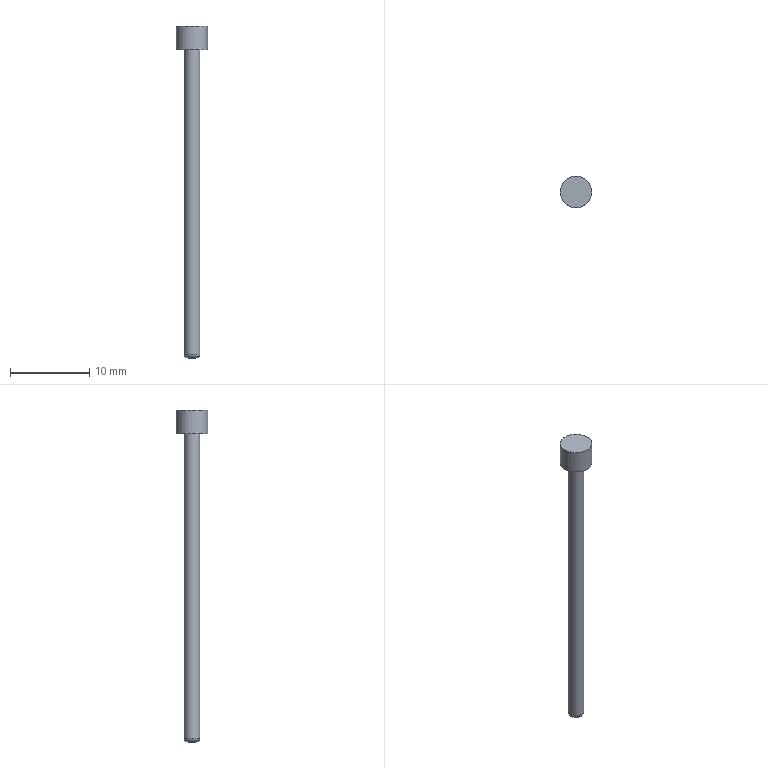Part | STEP file | gslz 2016.10.28-10_id2602_x_t | 1 solid | 6 faces | box 4 x 4 x 42 mm | volume 159.922 mm3 | plane 3 | cylinder 2 | torus 1 | commonest cylinder face diameters 2 x1 4 x1
STEP:
#1=CARTESIAN_POINT('',(0.,0.,0.));
#2=DIRECTION('',(0.,0.,1.));
#3=DIRECTION('',(1.,0.,0.));
#4=AXIS2_PLACEMENT_3D('',#1,#2,#3);
#5=CARTESIAN_POINT('',(1162.303,113.3,-12.5));
#6=VERTEX_POINT('',#5);
#7=CARTESIAN_POINT('',(1161.303,113.3,-12.5));
#8=DIRECTION('',(0.,0.,1.));
#9=DIRECTION('',(1.,0.,0.));
#10=AXIS2_PLACEMENT_3D('',#7,#8,#9);
#11=CIRCLE('',#10,1.);
#12=CARTESIAN_POINT('',(1161.303,113.3,-13.));
#13=DIRECTION('',(0.,0.,1.));
#14=DIRECTION('',(-1.,0.,0.));
#15=AXIS2_PLACEMENT_3D('',#12,#13,#14);
#16=CYLINDRICAL_SURFACE('',#15,1.);
#17=CARTESIAN_POINT('',(3.142,0.5));
#18=DIRECTION('',(1.,0.));
#19=VECTOR('',#18,1.);
#20=LINE('',#17,#19);
#21=(GEOMETRIC_REPRESENTATION_CONTEXT(2)PARAMETRIC_REPRESENTATION_CONTEXT()REPRESENTATION_CONTEXT('',''));
#22=DEFINITIONAL_REPRESENTATION('',(#20),#21);
#23=PCURVE('',#16,#22);
#24=CARTESIAN_POINT('',(1161.303,113.3,-12.5));
#25=DIRECTION('',(0.,0.,1.));
#26=DIRECTION('',(0.,-1.,0.));
#27=AXIS2_PLACEMENT_3D('',#24,#25,#26);
#28=TOROIDAL_SURFACE('',#27,0.5,0.5);
#29=CARTESIAN_POINT('',(1.571,6.283));
#30=DIRECTION('',(1.,0.));
#31=VECTOR('',#30,1.);
#32=LINE('',#29,#31);
#33=(GEOMETRIC_REPRESENTATION_CONTEXT(2)PARAMETRIC_REPRESENTATION_CONTEXT()REPRESENTATION_CONTEXT('',''));
#34=DEFINITIONAL_REPRESENTATION('',(#32),#33);
#35=PCURVE('',#28,#34);
#36=SURFACE_CURVE('',#11,(#23,#35),.PCURVE_S1.);
#37=EDGE_CURVE('',#6,#6,#36,.T.);
#38=ORIENTED_EDGE('',*,*,#37,.T.);
#39=CARTESIAN_POINT('',(1162.303,113.3,26.));
#40=VERTEX_POINT('',#39);
#41=CARTESIAN_POINT('',(1162.303,113.3,-12.5));
#42=CARTESIAN_POINT('',(1162.303,113.3,26.));
#43=B_SPLINE_CURVE_WITH_KNOTS('',1,(#41,#42),.UNSPECIFIED.,.F.,.F.,(2,2),(0.5,39.),.PIECEWISE_BEZIER_KNOTS.);
#44=CARTESIAN_POINT('',(9.425,0.));
#45=DIRECTION('',(0.,1.));
#46=VECTOR('',#45,1.);
#47=LINE('',#44,#46);
#48=(GEOMETRIC_REPRESENTATION_CONTEXT(2)PARAMETRIC_REPRESENTATION_CONTEXT()REPRESENTATION_CONTEXT('',''));
#49=DEFINITIONAL_REPRESENTATION('',(#47),#48);
#50=PCURVE('',#16,#49);
#51=CARTESIAN_POINT('',(3.142,0.));
#52=DIRECTION('',(0.,1.));
#53=VECTOR('',#52,1.);
#54=LINE('',#51,#53);
#55=(GEOMETRIC_REPRESENTATION_CONTEXT(2)PARAMETRIC_REPRESENTATION_CONTEXT()REPRESENTATION_CONTEXT('',''));
#56=DEFINITIONAL_REPRESENTATION('',(#54),#55);
#57=PCURVE('',#16,#56);
#58=SEAM_CURVE('',#43,(#50,#57),.PCURVE_S1.);
#59=EDGE_CURVE('',#6,#40,#58,.T.);
#60=ORIENTED_EDGE('',*,*,#59,.T.);
#61=CARTESIAN_POINT('',(1161.303,113.3,26.));
#62=DIRECTION('',(0.,0.,1.));
#63=DIRECTION('',(1.,0.,0.));
#64=AXIS2_PLACEMENT_3D('',#61,#62,#63);
#65=CIRCLE('',#64,1.);
#66=CARTESIAN_POINT('',(3.142,39.));
#67=DIRECTION('',(1.,0.));
#68=VECTOR('',#67,1.);
#69=LINE('',#66,#68);
#70=(GEOMETRIC_REPRESENTATION_CONTEXT(2)PARAMETRIC_REPRESENTATION_CONTEXT()REPRESENTATION_CONTEXT('',''));
#71=DEFINITIONAL_REPRESENTATION('',(#69),#70);
#72=PCURVE('',#16,#71);
#73=CARTESIAN_POINT('',(1161.303,113.3,26.));
#74=DIRECTION('',(0.,0.,1.));
#75=DIRECTION('',(-1.,0.,0.));
#76=AXIS2_PLACEMENT_3D('',#73,#74,#75);
#77=PLANE('',#76);
#78=CARTESIAN_POINT('',(0.,0.));
#79=DIRECTION('',(-1.,0.));
#80=AXIS2_PLACEMENT_2D('',#78,#79);
#81=CIRCLE('',#80,1.);
#82=(GEOMETRIC_REPRESENTATION_CONTEXT(2)PARAMETRIC_REPRESENTATION_CONTEXT()REPRESENTATION_CONTEXT('',''));
#83=DEFINITIONAL_REPRESENTATION('',(#81),#82);
#84=PCURVE('',#77,#83);
#85=SURFACE_CURVE('',#65,(#72,#84),.PCURVE_S1.);
#86=EDGE_CURVE('',#40,#40,#85,.T.);
#87=ORIENTED_EDGE('',*,*,#86,.F.);
#88=ORIENTED_EDGE('',*,*,#59,.F.);
#89=EDGE_LOOP('',(#38,#60,#87,#88));
#90=FACE_BOUND('',#89,.T.);
#91=ADVANCED_FACE('',(#90),#16,.T.);
#92=CARTESIAN_POINT('',(1161.803,113.3,-13.));
#93=VERTEX_POINT('',#92);
#94=CARTESIAN_POINT('',(1161.303,113.3,-13.));
#95=DIRECTION('',(0.,0.,-1.));
#96=DIRECTION('',(1.,0.,0.));
#97=AXIS2_PLACEMENT_3D('',#94,#95,#96);
#98=CIRCLE('',#97,0.5);
#99=CARTESIAN_POINT('',(1161.303,113.3,-13.));
#100=DIRECTION('',(0.,0.,1.));
#101=DIRECTION('',(-1.,0.,0.));
#102=AXIS2_PLACEMENT_3D('',#99,#100,#101);
#103=PLANE('',#102);
#104=CARTESIAN_POINT('',(-0.5,0.));
#105=CARTESIAN_POINT('',(-0.5,0.866));
#106=CARTESIAN_POINT('',(0.25,0.433));
#107=CARTESIAN_POINT('',(1.,0.));
#108=CARTESIAN_POINT('',(0.25,-0.433));
#109=CARTESIAN_POINT('',(-0.5,-0.866));
#110=CARTESIAN_POINT('',(-0.5,0.));
#111=(BOUNDED_CURVE()B_SPLINE_CURVE(2,(#104,#105,#106,#107,#108,#109,#110),.UNSPECIFIED.,.T.,.F.)B_SPLINE_CURVE_WITH_KNOTS((1,2,2,2,2,1),(-2.094,0.,2.094,4.189,6.283,8.378),.UNSPECIFIED.)CURVE()GEOMETRIC_REPRESENTATION_ITEM()RATIONAL_B_SPLINE_CURVE((1.,0.5,1.,0.5,1.,0.5,1.))REPRESENTATION_ITEM(''));
#112=(GEOMETRIC_REPRESENTATION_CONTEXT(2)PARAMETRIC_REPRESENTATION_CONTEXT()REPRESENTATION_CONTEXT('',''));
#113=DEFINITIONAL_REPRESENTATION('',(#111),#112);
#114=PCURVE('',#103,#113);
#115=CARTESIAN_POINT('',(7.854,4.712));
#116=DIRECTION('',(-1.,0.));
#117=VECTOR('',#116,1.);
#118=LINE('',#115,#117);
#119=(GEOMETRIC_REPRESENTATION_CONTEXT(2)PARAMETRIC_REPRESENTATION_CONTEXT()REPRESENTATION_CONTEXT('',''));
#120=DEFINITIONAL_REPRESENTATION('',(#118),#119);
#121=PCURVE('',#28,#120);
#122=SURFACE_CURVE('',#98,(#114,#121),.PCURVE_S1.);
#123=EDGE_CURVE('',#93,#93,#122,.T.);
#124=ORIENTED_EDGE('',*,*,#123,.T.);
#125=EDGE_LOOP('',(#124));
#126=FACE_BOUND('',#125,.T.);
#127=ADVANCED_FACE('',(#126),#103,.F.);
#128=CARTESIAN_POINT('',(1163.303,113.3,26.));
#129=VERTEX_POINT('',#128);
#130=CARTESIAN_POINT('',(1161.303,113.3,26.));
#131=DIRECTION('',(0.,0.,1.));
#132=DIRECTION('',(1.,0.,0.));
#133=AXIS2_PLACEMENT_3D('',#130,#131,#132);
#134=CIRCLE('',#133,2.);
#135=CARTESIAN_POINT('',(0.,0.));
#136=DIRECTION('',(-1.,0.));
#137=AXIS2_PLACEMENT_2D('',#135,#136);
#138=CIRCLE('',#137,2.);
#139=(GEOMETRIC_REPRESENTATION_CONTEXT(2)PARAMETRIC_REPRESENTATION_CONTEXT()REPRESENTATION_CONTEXT('',''));
#140=DEFINITIONAL_REPRESENTATION('',(#138),#139);
#141=PCURVE('',#77,#140);
#142=CARTESIAN_POINT('',(1161.303,113.3,29.));
#143=DIRECTION('',(0.,0.,-1.));
#144=DIRECTION('',(1.,0.,0.));
#145=AXIS2_PLACEMENT_3D('',#142,#143,#144);
#146=CYLINDRICAL_SURFACE('',#145,2.);
#147=CARTESIAN_POINT('',(6.283,3.));
#148=DIRECTION('',(-1.,0.));
#149=VECTOR('',#148,1.);
#150=LINE('',#147,#149);
#151=(GEOMETRIC_REPRESENTATION_CONTEXT(2)PARAMETRIC_REPRESENTATION_CONTEXT()REPRESENTATION_CONTEXT('',''));
#152=DEFINITIONAL_REPRESENTATION('',(#150),#151);
#153=PCURVE('',#146,#152);
#154=SURFACE_CURVE('',#134,(#141,#153),.PCURVE_S1.);
#155=EDGE_CURVE('',#129,#129,#154,.T.);
#156=ORIENTED_EDGE('',*,*,#155,.F.);
#157=EDGE_LOOP('',(#156));
#158=FACE_BOUND('',#157,.T.);
#159=ORIENTED_EDGE('',*,*,#86,.T.);
#160=EDGE_LOOP('',(#159));
#161=FACE_BOUND('',#160,.T.);
#162=ADVANCED_FACE('',(#158,#161),#77,.F.);
#163=CARTESIAN_POINT('',(1163.303,113.3,29.));
#164=VERTEX_POINT('',#163);
#165=CARTESIAN_POINT('',(1161.303,113.3,29.));
#166=DIRECTION('',(0.,0.,1.));
#167=DIRECTION('',(1.,0.,0.));
#168=AXIS2_PLACEMENT_3D('',#165,#166,#167);
#169=CIRCLE('',#168,2.);
#170=CARTESIAN_POINT('',(6.283,0.));
#171=DIRECTION('',(-1.,0.));
#172=VECTOR('',#171,1.);
#173=LINE('',#170,#172);
#174=(GEOMETRIC_REPRESENTATION_CONTEXT(2)PARAMETRIC_REPRESENTATION_CONTEXT()REPRESENTATION_CONTEXT('',''));
#175=DEFINITIONAL_REPRESENTATION('',(#173),#174);
#176=PCURVE('',#146,#175);
#177=CARTESIAN_POINT('',(1161.303,113.3,29.));
#178=DIRECTION('',(0.,0.,1.));
#179=DIRECTION('',(-1.,0.,0.));
#180=AXIS2_PLACEMENT_3D('',#177,#178,#179);
#181=PLANE('',#180);
#182=CARTESIAN_POINT('',(0.,0.));
#183=DIRECTION('',(-1.,0.));
#184=AXIS2_PLACEMENT_2D('',#182,#183);
#185=CIRCLE('',#184,2.);
#186=(GEOMETRIC_REPRESENTATION_CONTEXT(2)PARAMETRIC_REPRESENTATION_CONTEXT()REPRESENTATION_CONTEXT('',''));
#187=DEFINITIONAL_REPRESENTATION('',(#185),#186);
#188=PCURVE('',#181,#187);
#189=SURFACE_CURVE('',#169,(#176,#188),.PCURVE_S1.);
#190=EDGE_CURVE('',#164,#164,#189,.T.);
#191=ORIENTED_EDGE('',*,*,#190,.F.);
#192=CARTESIAN_POINT('',(1163.303,113.3,29.));
#193=CARTESIAN_POINT('',(1163.303,113.3,26.));
#194=B_SPLINE_CURVE_WITH_KNOTS('',1,(#192,#193),.UNSPECIFIED.,.F.,.F.,(2,2),(0.,3.),.PIECEWISE_BEZIER_KNOTS.);
#195=CARTESIAN_POINT('',(6.283,0.));
#196=DIRECTION('',(0.,1.));
#197=VECTOR('',#196,1.);
#198=LINE('',#195,#197);
#199=(GEOMETRIC_REPRESENTATION_CONTEXT(2)PARAMETRIC_REPRESENTATION_CONTEXT()REPRESENTATION_CONTEXT('',''));
#200=DEFINITIONAL_REPRESENTATION('',(#198),#199);
#201=PCURVE('',#146,#200);
#202=CARTESIAN_POINT('',(0.,0.));
#203=DIRECTION('',(0.,1.));
#204=VECTOR('',#203,1.);
#205=LINE('',#202,#204);
#206=(GEOMETRIC_REPRESENTATION_CONTEXT(2)PARAMETRIC_REPRESENTATION_CONTEXT()REPRESENTATION_CONTEXT('',''));
#207=DEFINITIONAL_REPRESENTATION('',(#205),#206);
#208=PCURVE('',#146,#207);
#209=SEAM_CURVE('',#194,(#201,#208),.PCURVE_S1.);
#210=EDGE_CURVE('',#164,#129,#209,.T.);
#211=ORIENTED_EDGE('',*,*,#210,.T.);
#212=ORIENTED_EDGE('',*,*,#155,.T.);
#213=ORIENTED_EDGE('',*,*,#210,.F.);
#214=EDGE_LOOP('',(#191,#211,#212,#213));
#215=FACE_BOUND('',#214,.T.);
#216=ADVANCED_FACE('',(#215),#146,.T.);
#217=ORIENTED_EDGE('',*,*,#190,.T.);
#218=EDGE_LOOP('',(#217));
#219=FACE_BOUND('',#218,.T.);
#220=ADVANCED_FACE('',(#219),#181,.T.);
#221=ORIENTED_EDGE('',*,*,#123,.F.);
#222=CARTESIAN_POINT('',(1161.803,113.3,-13.));
#223=CARTESIAN_POINT('',(1161.937,113.3,-13.));
#224=CARTESIAN_POINT('',(1162.067,113.3,-12.957));
#225=CARTESIAN_POINT('',(1162.179,113.3,-12.876));
#226=CARTESIAN_POINT('',(1162.26,113.3,-12.764));
#227=CARTESIAN_POINT('',(1162.303,113.3,-12.634));
#228=CARTESIAN_POINT('',(1162.303,113.3,-12.5));
#229=(BOUNDED_CURVE()B_SPLINE_CURVE(6,(#222,#223,#224,#225,#226,#227,#228),.UNSPECIFIED.,.F.,.F.)B_SPLINE_CURVE_WITH_KNOTS((7,7),(4.712,6.283),.PIECEWISE_BEZIER_KNOTS.)CURVE()GEOMETRIC_REPRESENTATION_ITEM()RATIONAL_B_SPLINE_CURVE((1.031,1.01,0.9979,0.994,0.9979,1.01,1.031))REPRESENTATION_ITEM(''));
#230=CARTESIAN_POINT('',(7.854,0.));
#231=DIRECTION('',(0.,1.));
#232=VECTOR('',#231,1.);
#233=LINE('',#230,#232);
#234=(GEOMETRIC_REPRESENTATION_CONTEXT(2)PARAMETRIC_REPRESENTATION_CONTEXT()REPRESENTATION_CONTEXT('',''));
#235=DEFINITIONAL_REPRESENTATION('',(#233),#234);
#236=PCURVE('',#28,#235);
#237=CARTESIAN_POINT('',(1.571,0.));
#238=DIRECTION('',(0.,1.));
#239=VECTOR('',#238,1.);
#240=LINE('',#237,#239);
#241=(GEOMETRIC_REPRESENTATION_CONTEXT(2)PARAMETRIC_REPRESENTATION_CONTEXT()REPRESENTATION_CONTEXT('',''));
#242=DEFINITIONAL_REPRESENTATION('',(#240),#241);
#243=PCURVE('',#28,#242);
#244=SEAM_CURVE('',#229,(#236,#243),.PCURVE_S1.);
#245=EDGE_CURVE('',#93,#6,#244,.T.);
#246=ORIENTED_EDGE('',*,*,#245,.T.);
#247=ORIENTED_EDGE('',*,*,#37,.F.);
#248=ORIENTED_EDGE('',*,*,#245,.F.);
#249=EDGE_LOOP('',(#221,#246,#247,#248));
#250=FACE_BOUND('',#249,.T.);
#251=ADVANCED_FACE('',(#250),#28,.T.);
#252=CLOSED_SHELL('',(#91,#127,#162,#216,#220,#251));
#253=MANIFOLD_SOLID_BREP('',#252);
#254=(LENGTH_UNIT()NAMED_UNIT(*)SI_UNIT(.MILLI.,.METRE.));
#255=UNCERTAINTY_MEASURE_WITH_UNIT(LENGTH_MEASURE(0.00001),#254,'','');
#256=(NAMED_UNIT(*)PLANE_ANGLE_UNIT()SI_UNIT($,.RADIAN.));
#257=(NAMED_UNIT(*)SI_UNIT($,.STERADIAN.)SOLID_ANGLE_UNIT());
#258=(GEOMETRIC_REPRESENTATION_CONTEXT(3)GLOBAL_UNCERTAINTY_ASSIGNED_CONTEXT((#255))GLOBAL_UNIT_ASSIGNED_CONTEXT((#254,#256,#257))REPRESENTATION_CONTEXT('',''));
#259=ADVANCED_BREP_SHAPE_REPRESENTATION('',(#4,#253),#258);